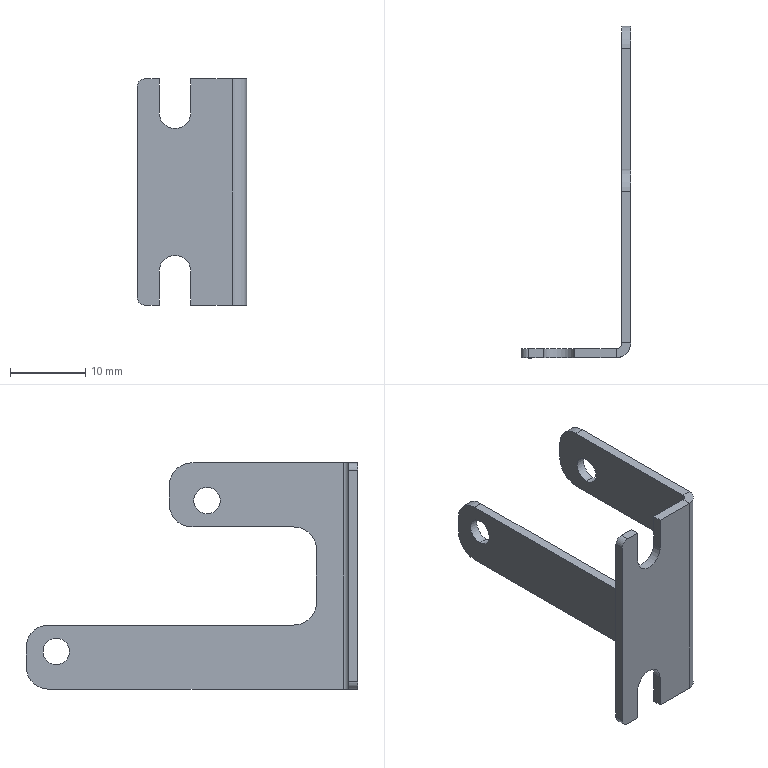Part | SolidWorks | features ICE 3, Fillet 2, EdgeFlange 1, FlatPattern 1, MirrorPattern 1, SMBaseFlange 1, SheetMetal 1 | 1 solid | 38 faces | box 14.5 x 44 x 30 mm | volume 1158 mm3 | plane 22 | cylinder 16 | commonest cylinder face diameters 6 x6 3.5 x4 2 x2 4.2 x2 1.473 x1 3.873 x1
STEP:
#1=CARTESIAN_POINT('',(-1.2,18.,-11.75));
#2=VERTEX_POINT('',#1);
#3=CARTESIAN_POINT('',(-1.2,18.,-8.25));
#4=VERTEX_POINT('',#3);
#5=CARTESIAN_POINT('',(-1.2,18.,-10.));
#6=DIRECTION('',(-1.,0.,0.));
#7=DIRECTION('',(0.,0.,1.));
#8=AXIS2_PLACEMENT_3D('',#5,#6,#7);
#9=CIRCLE('',#8,1.75);
#10=EDGE_CURVE('',#2,#4,#9,.T.);
#11=ORIENTED_EDGE('',*,*,#10,.T.);
#12=CARTESIAN_POINT('',(0.,18.,-8.25));
#13=VERTEX_POINT('',#12);
#14=CARTESIAN_POINT('',(-10.,18.,-8.25));
#15=DIRECTION('',(1.,0.,0.));
#16=VECTOR('',#15,1000.);
#17=LINE('',#14,#16);
#18=EDGE_CURVE('',#4,#13,#17,.T.);
#19=ORIENTED_EDGE('',*,*,#18,.T.);
#20=CARTESIAN_POINT('',(0.,18.,-11.75));
#21=VERTEX_POINT('',#20);
#22=CARTESIAN_POINT('',(0.,18.,-10.));
#23=DIRECTION('',(1.,0.,0.));
#24=DIRECTION('',(0.,0.,-1.));
#25=AXIS2_PLACEMENT_3D('',#22,#23,#24);
#26=CIRCLE('',#25,1.75);
#27=EDGE_CURVE('',#13,#21,#26,.T.);
#28=ORIENTED_EDGE('',*,*,#27,.T.);
#29=CARTESIAN_POINT('',(-10.,18.,-11.75));
#30=DIRECTION('',(1.,0.,0.));
#31=VECTOR('',#30,1000.);
#32=LINE('',#29,#31);
#33=EDGE_CURVE('',#2,#21,#32,.T.);
#34=ORIENTED_EDGE('',*,*,#33,.F.);
#35=EDGE_LOOP('',(#11,#19,#28,#34));
#36=FACE_OUTER_BOUND('',#35,.T.);
#37=CARTESIAN_POINT('',(-10.,18.,-10.));
#38=DIRECTION('',(1.,0.,0.));
#39=DIRECTION('',(0.,0.,-1.));
#40=AXIS2_PLACEMENT_3D('',#37,#38,#39);
#41=CYLINDRICAL_SURFACE('',#40,1.75);
#42=ADVANCED_FACE('',(#36),#41,.F.);
#43=CARTESIAN_POINT('',(-1.2,-2.,8.25));
#44=VERTEX_POINT('',#43);
#45=CARTESIAN_POINT('',(-1.2,-2.,11.75));
#46=VERTEX_POINT('',#45);
#47=CARTESIAN_POINT('',(-1.2,-2.,10.));
#48=DIRECTION('',(-1.,0.,0.));
#49=DIRECTION('',(0.,0.,1.));
#50=AXIS2_PLACEMENT_3D('',#47,#48,#49);
#51=CIRCLE('',#50,1.75);
#52=EDGE_CURVE('',#44,#46,#51,.T.);
#53=ORIENTED_EDGE('',*,*,#52,.T.);
#54=CARTESIAN_POINT('',(0.,-2.,11.75));
#55=VERTEX_POINT('',#54);
#56=CARTESIAN_POINT('',(-10.,-2.,11.75));
#57=DIRECTION('',(1.,0.,0.));
#58=VECTOR('',#57,1000.);
#59=LINE('',#56,#58);
#60=EDGE_CURVE('',#46,#55,#59,.T.);
#61=ORIENTED_EDGE('',*,*,#60,.T.);
#62=CARTESIAN_POINT('',(0.,-2.,8.25));
#63=VERTEX_POINT('',#62);
#64=CARTESIAN_POINT('',(0.,-2.,10.));
#65=DIRECTION('',(1.,0.,0.));
#66=DIRECTION('',(0.,0.,-1.));
#67=AXIS2_PLACEMENT_3D('',#64,#65,#66);
#68=CIRCLE('',#67,1.75);
#69=EDGE_CURVE('',#55,#63,#68,.T.);
#70=ORIENTED_EDGE('',*,*,#69,.T.);
#71=CARTESIAN_POINT('',(-10.,-2.,8.25));
#72=DIRECTION('',(1.,0.,0.));
#73=VECTOR('',#72,1000.);
#74=LINE('',#71,#73);
#75=EDGE_CURVE('',#44,#63,#74,.T.);
#76=ORIENTED_EDGE('',*,*,#75,.F.);
#77=EDGE_LOOP('',(#53,#61,#70,#76));
#78=FACE_OUTER_BOUND('',#77,.T.);
#79=CARTESIAN_POINT('',(-10.,-2.,10.));
#80=DIRECTION('',(1.,0.,0.));
#81=DIRECTION('',(0.,0.,-1.));
#82=AXIS2_PLACEMENT_3D('',#79,#80,#81);
#83=CYLINDRICAL_SURFACE('',#82,1.75);
#84=ADVANCED_FACE('',(#78),#83,.F.);
#85=CARTESIAN_POINT('',(-7.4,-20.8,15.));
#86=VERTEX_POINT('',#85);
#87=CARTESIAN_POINT('',(-1.937,-20.8,15.));
#88=VERTEX_POINT('',#87);
#89=CARTESIAN_POINT('',(-1.2,-20.8,15.));
#90=DIRECTION('',(1.,0.,0.));
#91=VECTOR('',#90,1000.);
#92=LINE('',#89,#91);
#93=EDGE_CURVE('',#86,#88,#92,.T.);
#94=ORIENTED_EDGE('',*,*,#93,.F.);
#95=CARTESIAN_POINT('',(-7.4,-22.,15.));
#96=VERTEX_POINT('',#95);
#97=CARTESIAN_POINT('',(-7.4,-30.8,15.));
#98=DIRECTION('',(0.,1.,0.));
#99=VECTOR('',#98,1000.);
#100=LINE('',#97,#99);
#101=EDGE_CURVE('',#96,#86,#100,.T.);
#102=ORIENTED_EDGE('',*,*,#101,.F.);
#103=CARTESIAN_POINT('',(-1.937,-22.,15.));
#104=VERTEX_POINT('',#103);
#105=CARTESIAN_POINT('',(-1.2,-22.,15.));
#106=DIRECTION('',(1.,0.,0.));
#107=VECTOR('',#106,1000.);
#108=LINE('',#105,#107);
#109=EDGE_CURVE('',#96,#104,#108,.T.);
#110=ORIENTED_EDGE('',*,*,#109,.T.);
#111=CARTESIAN_POINT('',(-1.937,-20.8,15.));
#112=DIRECTION('',(0.,-1.,0.));
#113=VECTOR('',#112,1000.);
#114=LINE('',#111,#113);
#115=EDGE_CURVE('',#88,#104,#114,.T.);
#116=ORIENTED_EDGE('',*,*,#115,.F.);
#117=EDGE_LOOP('',(#94,#102,#110,#116));
#118=FACE_OUTER_BOUND('',#117,.T.);
#119=CARTESIAN_POINT('',(-1.2,-22.,15.));
#120=DIRECTION('',(0.,0.,1.));
#121=DIRECTION('',(1.,0.,0.));
#122=AXIS2_PLACEMENT_3D('',#119,#120,#121);
#123=PLANE('',#122);
#124=ADVANCED_FACE('',(#118),#123,.T.);
#125=CARTESIAN_POINT('',(-13.5,-22.,15.));
#126=VERTEX_POINT('',#125);
#127=CARTESIAN_POINT('',(-11.6,-22.,15.));
#128=VERTEX_POINT('',#127);
#129=CARTESIAN_POINT('',(-1.2,-22.,15.));
#130=DIRECTION('',(1.,0.,0.));
#131=VECTOR('',#130,1000.);
#132=LINE('',#129,#131);
#133=EDGE_CURVE('',#126,#128,#132,.T.);
#134=ORIENTED_EDGE('',*,*,#133,.T.);
#135=CARTESIAN_POINT('',(-11.6,-20.8,15.));
#136=VERTEX_POINT('',#135);
#137=CARTESIAN_POINT('',(-11.6,-30.8,15.));
#138=DIRECTION('',(0.,1.,0.));
#139=VECTOR('',#138,1000.);
#140=LINE('',#137,#139);
#141=EDGE_CURVE('',#128,#136,#140,.T.);
#142=ORIENTED_EDGE('',*,*,#141,.T.);
#143=CARTESIAN_POINT('',(-13.5,-20.8,15.));
#144=VERTEX_POINT('',#143);
#145=CARTESIAN_POINT('',(-1.2,-20.8,15.));
#146=DIRECTION('',(1.,0.,0.));
#147=VECTOR('',#146,1000.);
#148=LINE('',#145,#147);
#149=EDGE_CURVE('',#144,#136,#148,.T.);
#150=ORIENTED_EDGE('',*,*,#149,.F.);
#151=CARTESIAN_POINT('',(-13.5,-22.,15.));
#152=DIRECTION('',(0.,-1.,0.));
#153=VECTOR('',#152,1000.);
#154=LINE('',#151,#153);
#155=EDGE_CURVE('',#144,#126,#154,.T.);
#156=ORIENTED_EDGE('',*,*,#155,.T.);
#157=EDGE_LOOP('',(#134,#142,#150,#156));
#158=FACE_OUTER_BOUND('',#157,.T.);
#159=CARTESIAN_POINT('',(-1.2,-22.,15.));
#160=DIRECTION('',(0.,0.,1.));
#161=DIRECTION('',(1.,0.,0.));
#162=AXIS2_PLACEMENT_3D('',#159,#160,#161);
#163=PLANE('',#162);
#164=ADVANCED_FACE('',(#158),#163,.T.);
#165=ORIENTED_EDGE('',*,*,#109,.F.);
#166=CARTESIAN_POINT('',(-7.4,-22.,10.5));
#167=VERTEX_POINT('',#166);
#168=CARTESIAN_POINT('',(-7.4,-22.,15.));
#169=DIRECTION('',(0.,0.,-1.));
#170=VECTOR('',#169,1000.);
#171=LINE('',#168,#170);
#172=EDGE_CURVE('',#96,#167,#171,.T.);
#173=ORIENTED_EDGE('',*,*,#172,.T.);
#174=CARTESIAN_POINT('',(-11.6,-22.,10.5));
#175=VERTEX_POINT('',#174);
#176=CARTESIAN_POINT('',(-9.5,-22.,10.5));
#177=DIRECTION('',(0.,1.,0.));
#178=DIRECTION('',(1.,0.,0.));
#179=AXIS2_PLACEMENT_3D('',#176,#177,#178);
#180=CIRCLE('',#179,2.1);
#181=EDGE_CURVE('',#167,#175,#180,.T.);
#182=ORIENTED_EDGE('',*,*,#181,.T.);
#183=CARTESIAN_POINT('',(-11.6,-22.,15.));
#184=DIRECTION('',(0.,0.,1.));
#185=VECTOR('',#184,1000.);
#186=LINE('',#183,#185);
#187=EDGE_CURVE('',#175,#128,#186,.T.);
#188=ORIENTED_EDGE('',*,*,#187,.T.);
#189=ORIENTED_EDGE('',*,*,#133,.F.);
#190=CARTESIAN_POINT('',(-14.5,-22.,14.));
#191=VERTEX_POINT('',#190);
#192=CARTESIAN_POINT('',(-13.5,-22.,14.));
#193=DIRECTION('',(0.,-1.,0.));
#194=DIRECTION('',(1.,0.,0.));
#195=AXIS2_PLACEMENT_3D('',#192,#193,#194);
#196=CIRCLE('',#195,1.);
#197=EDGE_CURVE('',#126,#191,#196,.T.);
#198=ORIENTED_EDGE('',*,*,#197,.T.);
#199=CARTESIAN_POINT('',(-14.5,-22.,-14.));
#200=VERTEX_POINT('',#199);
#201=CARTESIAN_POINT('',(-14.5,-22.,15.));
#202=DIRECTION('',(0.,0.,1.));
#203=VECTOR('',#202,1000.);
#204=LINE('',#201,#203);
#205=EDGE_CURVE('',#200,#191,#204,.T.);
#206=ORIENTED_EDGE('',*,*,#205,.F.);
#207=CARTESIAN_POINT('',(-13.5,-22.,-15.));
#208=VERTEX_POINT('',#207);
#209=CARTESIAN_POINT('',(-13.5,-22.,-14.));
#210=DIRECTION('',(0.,-1.,0.));
#211=DIRECTION('',(1.,0.,0.));
#212=AXIS2_PLACEMENT_3D('',#209,#210,#211);
#213=CIRCLE('',#212,1.);
#214=EDGE_CURVE('',#200,#208,#213,.T.);
#215=ORIENTED_EDGE('',*,*,#214,.T.);
#216=CARTESIAN_POINT('',(-11.6,-22.,-15.));
#217=VERTEX_POINT('',#216);
#218=CARTESIAN_POINT('',(-14.5,-22.,-15.));
#219=DIRECTION('',(-1.,0.,0.));
#220=VECTOR('',#219,1000.);
#221=LINE('',#218,#220);
#222=EDGE_CURVE('',#217,#208,#221,.T.);
#223=ORIENTED_EDGE('',*,*,#222,.F.);
#224=CARTESIAN_POINT('',(-11.6,-22.,-10.5));
#225=VERTEX_POINT('',#224);
#226=CARTESIAN_POINT('',(-11.6,-22.,15.));
#227=DIRECTION('',(0.,0.,-1.));
#228=VECTOR('',#227,1000.);
#229=LINE('',#226,#228);
#230=EDGE_CURVE('',#225,#217,#229,.T.);
#231=ORIENTED_EDGE('',*,*,#230,.F.);
#232=CARTESIAN_POINT('',(-7.4,-22.,-10.5));
#233=VERTEX_POINT('',#232);
#234=CARTESIAN_POINT('',(-9.5,-22.,-10.5));
#235=DIRECTION('',(0.,-1.,0.));
#236=DIRECTION('',(1.,0.,0.));
#237=AXIS2_PLACEMENT_3D('',#234,#235,#236);
#238=CIRCLE('',#237,2.1);
#239=EDGE_CURVE('',#233,#225,#238,.T.);
#240=ORIENTED_EDGE('',*,*,#239,.F.);
#241=CARTESIAN_POINT('',(-7.4,-22.,-15.));
#242=VERTEX_POINT('',#241);
#243=CARTESIAN_POINT('',(-7.4,-22.,15.));
#244=DIRECTION('',(0.,0.,1.));
#245=VECTOR('',#244,1000.);
#246=LINE('',#243,#245);
#247=EDGE_CURVE('',#242,#233,#246,.T.);
#248=ORIENTED_EDGE('',*,*,#247,.F.);
#249=CARTESIAN_POINT('',(-1.937,-22.,-15.));
#250=VERTEX_POINT('',#249);
#251=CARTESIAN_POINT('',(-14.5,-22.,-15.));
#252=DIRECTION('',(-1.,0.,0.));
#253=VECTOR('',#252,1000.);
#254=LINE('',#251,#253);
#255=EDGE_CURVE('',#250,#242,#254,.T.);
#256=ORIENTED_EDGE('',*,*,#255,.F.);
#257=CARTESIAN_POINT('',(-1.937,-22.,15.));
#258=DIRECTION('',(0.,0.,1.));
#259=VECTOR('',#258,1000.);
#260=LINE('',#257,#259);
#261=EDGE_CURVE('',#250,#104,#260,.T.);
#262=ORIENTED_EDGE('',*,*,#261,.T.);
#263=EDGE_LOOP('',(#165,#173,#182,#188,#189,#198,#206,#215,#223,#231,#240,#248,#256,#262));
#264=FACE_OUTER_BOUND('',#263,.T.);
#265=CARTESIAN_POINT('',(-1.2,-22.,15.));
#266=DIRECTION('',(0.,-1.,0.));
#267=DIRECTION('',(1.,0.,0.));
#268=AXIS2_PLACEMENT_3D('',#265,#266,#267);
#269=PLANE('',#268);
#270=ADVANCED_FACE('',(#264),#269,.T.);
#271=CARTESIAN_POINT('',(-7.4,-20.8,10.5));
#272=VERTEX_POINT('',#271);
#273=CARTESIAN_POINT('',(-7.4,-20.8,15.));
#274=DIRECTION('',(0.,0.,1.));
#275=VECTOR('',#274,1000.);
#276=LINE('',#273,#275);
#277=EDGE_CURVE('',#272,#86,#276,.T.);
#278=ORIENTED_EDGE('',*,*,#277,.T.);
#279=ORIENTED_EDGE('',*,*,#93,.T.);
#280=CARTESIAN_POINT('',(-1.937,-20.8,-15.));
#281=VERTEX_POINT('',#280);
#282=CARTESIAN_POINT('',(-1.937,-20.8,-15.));
#283=DIRECTION('',(0.,0.,1.));
#284=VECTOR('',#283,1000.);
#285=LINE('',#282,#284);
#286=EDGE_CURVE('',#281,#88,#285,.T.);
#287=ORIENTED_EDGE('',*,*,#286,.F.);
#288=CARTESIAN_POINT('',(-7.4,-20.8,-15.));
#289=VERTEX_POINT('',#288);
#290=CARTESIAN_POINT('',(-1.2,-20.8,-15.));
#291=DIRECTION('',(-1.,0.,0.));
#292=VECTOR('',#291,1000.);
#293=LINE('',#290,#292);
#294=EDGE_CURVE('',#281,#289,#293,.T.);
#295=ORIENTED_EDGE('',*,*,#294,.T.);
#296=CARTESIAN_POINT('',(-7.4,-20.8,-10.5));
#297=VERTEX_POINT('',#296);
#298=CARTESIAN_POINT('',(-7.4,-20.8,-15.));
#299=DIRECTION('',(0.,0.,-1.));
#300=VECTOR('',#299,1000.);
#301=LINE('',#298,#300);
#302=EDGE_CURVE('',#297,#289,#301,.T.);
#303=ORIENTED_EDGE('',*,*,#302,.F.);
#304=CARTESIAN_POINT('',(-11.6,-20.8,-10.5));
#305=VERTEX_POINT('',#304);
#306=CARTESIAN_POINT('',(-9.5,-20.8,-10.5));
#307=DIRECTION('',(0.,1.,0.));
#308=DIRECTION('',(1.,0.,0.));
#309=AXIS2_PLACEMENT_3D('',#306,#307,#308);
#310=CIRCLE('',#309,2.1);
#311=EDGE_CURVE('',#305,#297,#310,.T.);
#312=ORIENTED_EDGE('',*,*,#311,.F.);
#313=CARTESIAN_POINT('',(-11.6,-20.8,-15.));
#314=VERTEX_POINT('',#313);
#315=CARTESIAN_POINT('',(-11.6,-20.8,-15.));
#316=DIRECTION('',(0.,0.,1.));
#317=VECTOR('',#316,1000.);
#318=LINE('',#315,#317);
#319=EDGE_CURVE('',#314,#305,#318,.T.);
#320=ORIENTED_EDGE('',*,*,#319,.F.);
#321=CARTESIAN_POINT('',(-13.5,-20.8,-15.));
#322=VERTEX_POINT('',#321);
#323=CARTESIAN_POINT('',(-1.2,-20.8,-15.));
#324=DIRECTION('',(-1.,0.,0.));
#325=VECTOR('',#324,1000.);
#326=LINE('',#323,#325);
#327=EDGE_CURVE('',#314,#322,#326,.T.);
#328=ORIENTED_EDGE('',*,*,#327,.T.);
#329=CARTESIAN_POINT('',(-14.5,-20.8,-14.));
#330=VERTEX_POINT('',#329);
#331=CARTESIAN_POINT('',(-13.5,-20.8,-14.));
#332=DIRECTION('',(0.,1.,0.));
#333=DIRECTION('',(1.,0.,0.));
#334=AXIS2_PLACEMENT_3D('',#331,#332,#333);
#335=CIRCLE('',#334,1.);
#336=EDGE_CURVE('',#322,#330,#335,.T.);
#337=ORIENTED_EDGE('',*,*,#336,.T.);
#338=CARTESIAN_POINT('',(-14.5,-20.8,14.));
#339=VERTEX_POINT('',#338);
#340=CARTESIAN_POINT('',(-14.5,-20.8,15.));
#341=DIRECTION('',(0.,0.,1.));
#342=VECTOR('',#341,1000.);
#343=LINE('',#340,#342);
#344=EDGE_CURVE('',#330,#339,#343,.T.);
#345=ORIENTED_EDGE('',*,*,#344,.T.);
#346=CARTESIAN_POINT('',(-13.5,-20.8,14.));
#347=DIRECTION('',(0.,1.,0.));
#348=DIRECTION('',(1.,0.,0.));
#349=AXIS2_PLACEMENT_3D('',#346,#347,#348);
#350=CIRCLE('',#349,1.);
#351=EDGE_CURVE('',#339,#144,#350,.T.);
#352=ORIENTED_EDGE('',*,*,#351,.T.);
#353=ORIENTED_EDGE('',*,*,#149,.T.);
#354=CARTESIAN_POINT('',(-11.6,-20.8,10.5));
#355=VERTEX_POINT('',#354);
#356=CARTESIAN_POINT('',(-11.6,-20.8,15.));
#357=DIRECTION('',(0.,0.,-1.));
#358=VECTOR('',#357,1000.);
#359=LINE('',#356,#358);
#360=EDGE_CURVE('',#136,#355,#359,.T.);
#361=ORIENTED_EDGE('',*,*,#360,.T.);
#362=CARTESIAN_POINT('',(-9.5,-20.8,10.5));
#363=DIRECTION('',(0.,-1.,0.));
#364=DIRECTION('',(1.,0.,0.));
#365=AXIS2_PLACEMENT_3D('',#362,#363,#364);
#366=CIRCLE('',#365,2.1);
#367=EDGE_CURVE('',#355,#272,#366,.T.);
#368=ORIENTED_EDGE('',*,*,#367,.T.);
#369=EDGE_LOOP('',(#278,#279,#287,#295,#303,#312,#320,#328,#337,#345,#352,#353,#361,#368));
#370=FACE_OUTER_BOUND('',#369,.T.);
#371=CARTESIAN_POINT('',(-1.2,-20.8,15.));
#372=DIRECTION('',(0.,-1.,0.));
#373=DIRECTION('',(1.,0.,0.));
#374=AXIS2_PLACEMENT_3D('',#371,#372,#373);
#375=PLANE('',#374);
#376=ADVANCED_FACE('',(#370),#375,.F.);
#377=CARTESIAN_POINT('',(-7.4,-30.8,-15.));
#378=DIRECTION('',(0.,1.,0.));
#379=VECTOR('',#378,1000.);
#380=LINE('',#377,#379);
#381=EDGE_CURVE('',#242,#289,#380,.T.);
#382=ORIENTED_EDGE('',*,*,#381,.T.);
#383=ORIENTED_EDGE('',*,*,#294,.F.);
#384=CARTESIAN_POINT('',(-1.937,-22.,-15.));
#385=DIRECTION('',(0.,-1.,0.));
#386=VECTOR('',#385,1000.);
#387=LINE('',#384,#386);
#388=EDGE_CURVE('',#281,#250,#387,.T.);
#389=ORIENTED_EDGE('',*,*,#388,.T.);
#390=ORIENTED_EDGE('',*,*,#255,.T.);
#391=EDGE_LOOP('',(#382,#383,#389,#390));
#392=FACE_OUTER_BOUND('',#391,.T.);
#393=CARTESIAN_POINT('',(-14.5,-22.,-15.));
#394=DIRECTION('',(0.,0.,-1.));
#395=DIRECTION('',(-1.,0.,0.));
#396=AXIS2_PLACEMENT_3D('',#393,#394,#395);
#397=PLANE('',#396);
#398=ADVANCED_FACE('',(#392),#397,.T.);
#399=CARTESIAN_POINT('',(-1.2,0.,15.));
#400=VERTEX_POINT('',#399);
#401=CARTESIAN_POINT('',(-1.2,-20.063,15.));
#402=VERTEX_POINT('',#401);
#403=CARTESIAN_POINT('',(-1.2,-22.,15.));
#404=DIRECTION('',(0.,-1.,0.));
#405=VECTOR('',#404,1000.);
#406=LINE('',#403,#405);
#407=EDGE_CURVE('',#400,#402,#406,.T.);
#408=ORIENTED_EDGE('',*,*,#407,.T.);
#409=CARTESIAN_POINT('',(0.,-20.063,15.));
#410=VERTEX_POINT('',#409);
#411=CARTESIAN_POINT('',(-1.2,-20.063,15.));
#412=DIRECTION('',(1.,0.,0.));
#413=VECTOR('',#412,1000.);
#414=LINE('',#411,#413);
#415=EDGE_CURVE('',#402,#410,#414,.T.);
#416=ORIENTED_EDGE('',*,*,#415,.T.);
#417=CARTESIAN_POINT('',(0.,0.,15.));
#418=VERTEX_POINT('',#417);
#419=CARTESIAN_POINT('',(0.,-22.,15.));
#420=DIRECTION('',(0.,-1.,0.));
#421=VECTOR('',#420,1000.);
#422=LINE('',#419,#421);
#423=EDGE_CURVE('',#418,#410,#422,.T.);
#424=ORIENTED_EDGE('',*,*,#423,.F.);
#425=CARTESIAN_POINT('',(-1.2,0.,15.));
#426=DIRECTION('',(-1.,0.,0.));
#427=VECTOR('',#426,1000.);
#428=LINE('',#425,#427);
#429=EDGE_CURVE('',#418,#400,#428,.T.);
#430=ORIENTED_EDGE('',*,*,#429,.T.);
#431=EDGE_LOOP('',(#408,#416,#424,#430));
#432=FACE_OUTER_BOUND('',#431,.T.);
#433=CARTESIAN_POINT('',(-1.2,-22.,15.));
#434=DIRECTION('',(0.,0.,1.));
#435=DIRECTION('',(1.,0.,0.));
#436=AXIS2_PLACEMENT_3D('',#433,#434,#435);
#437=PLANE('',#436);
#438=ADVANCED_FACE('',(#432),#437,.T.);
#439=ORIENTED_EDGE('',*,*,#10,.F.);
#440=CARTESIAN_POINT('',(-1.2,18.,-10.));
#441=DIRECTION('',(-1.,0.,0.));
#442=DIRECTION('',(0.,0.,1.));
#443=AXIS2_PLACEMENT_3D('',#440,#441,#442);
#444=CIRCLE('',#443,1.75);
#445=EDGE_CURVE('',#4,#2,#444,.T.);
#446=ORIENTED_EDGE('',*,*,#445,.F.);
#447=EDGE_LOOP('',(#439,#446));
#448=FACE_BOUND('',#447,.T.);
#449=ORIENTED_EDGE('',*,*,#52,.F.);
#450=CARTESIAN_POINT('',(-1.2,-2.,10.));
#451=DIRECTION('',(-1.,0.,0.));
#452=DIRECTION('',(0.,0.,1.));
#453=AXIS2_PLACEMENT_3D('',#450,#451,#452);
#454=CIRCLE('',#453,1.75);
#455=EDGE_CURVE('',#46,#44,#454,.T.);
#456=ORIENTED_EDGE('',*,*,#455,.F.);
#457=EDGE_LOOP('',(#449,#456));
#458=FACE_BOUND('',#457,.T.);
#459=CARTESIAN_POINT('',(-1.2,-20.063,-15.));
#460=VERTEX_POINT('',#459);
#461=CARTESIAN_POINT('',(-1.2,19.,-15.));
#462=VERTEX_POINT('',#461);
#463=CARTESIAN_POINT('',(-1.2,-22.,-15.));
#464=DIRECTION('',(0.,1.,0.));
#465=VECTOR('',#464,1000.);
#466=LINE('',#463,#465);
#467=EDGE_CURVE('',#460,#462,#466,.T.);
#468=ORIENTED_EDGE('',*,*,#467,.F.);
#469=CARTESIAN_POINT('',(-1.2,-20.063,15.));
#470=DIRECTION('',(0.,0.,-1.));
#471=VECTOR('',#470,1000.);
#472=LINE('',#469,#471);
#473=EDGE_CURVE('',#402,#460,#472,.T.);
#474=ORIENTED_EDGE('',*,*,#473,.F.);
#475=ORIENTED_EDGE('',*,*,#407,.F.);
#476=CARTESIAN_POINT('',(-1.2,3.,12.));
#477=VERTEX_POINT('',#476);
#478=CARTESIAN_POINT('',(-1.2,0.,12.));
#479=DIRECTION('',(-1.,0.,0.));
#480=DIRECTION('',(0.,0.,1.));
#481=AXIS2_PLACEMENT_3D('',#478,#479,#480);
#482=CIRCLE('',#481,3.);
#483=EDGE_CURVE('',#400,#477,#482,.T.);
#484=ORIENTED_EDGE('',*,*,#483,.T.);
#485=CARTESIAN_POINT('',(-1.2,3.,9.5));
#486=VERTEX_POINT('',#485);
#487=CARTESIAN_POINT('',(-1.2,3.,6.5));
#488=DIRECTION('',(0.,0.,-1.));
#489=VECTOR('',#488,1000.);
#490=LINE('',#487,#489);
#491=EDGE_CURVE('',#477,#486,#490,.T.);
#492=ORIENTED_EDGE('',*,*,#491,.T.);
#493=CARTESIAN_POINT('',(-1.2,0.,6.5));
#494=VERTEX_POINT('',#493);
#495=CARTESIAN_POINT('',(-1.2,0.,9.5));
#496=DIRECTION('',(-1.,0.,0.));
#497=DIRECTION('',(0.,0.,1.));
#498=AXIS2_PLACEMENT_3D('',#495,#496,#497);
#499=CIRCLE('',#498,3.);
#500=EDGE_CURVE('',#486,#494,#499,.T.);
#501=ORIENTED_EDGE('',*,*,#500,.T.);
#502=CARTESIAN_POINT('',(-1.2,-13.5,6.5));
#503=VERTEX_POINT('',#502);
#504=CARTESIAN_POINT('',(-1.2,3.,6.5));
#505=DIRECTION('',(0.,-1.,0.));
#506=VECTOR('',#505,1000.);
#507=LINE('',#504,#506);
#508=EDGE_CURVE('',#494,#503,#507,.T.);
#509=ORIENTED_EDGE('',*,*,#508,.T.);
#510=CARTESIAN_POINT('',(-1.2,-16.5,3.5));
#511=VERTEX_POINT('',#510);
#512=CARTESIAN_POINT('',(-1.2,-13.5,3.5));
#513=DIRECTION('',(1.,0.,0.));
#514=DIRECTION('',(0.,0.,1.));
#515=AXIS2_PLACEMENT_3D('',#512,#513,#514);
#516=CIRCLE('',#515,3.);
#517=EDGE_CURVE('',#503,#511,#516,.T.);
#518=ORIENTED_EDGE('',*,*,#517,.T.);
#519=CARTESIAN_POINT('',(-1.2,-16.5,-3.5));
#520=VERTEX_POINT('',#519);
#521=CARTESIAN_POINT('',(-1.2,-16.5,-6.5));
#522=DIRECTION('',(0.,0.,-1.));
#523=VECTOR('',#522,1000.);
#524=LINE('',#521,#523);
#525=EDGE_CURVE('',#511,#520,#524,.T.);
#526=ORIENTED_EDGE('',*,*,#525,.T.);
#527=CARTESIAN_POINT('',(-1.2,-13.5,-6.5));
#528=VERTEX_POINT('',#527);
#529=CARTESIAN_POINT('',(-1.2,-13.5,-3.5));
#530=DIRECTION('',(1.,0.,0.));
#531=DIRECTION('',(0.,0.,1.));
#532=AXIS2_PLACEMENT_3D('',#529,#530,#531);
#533=CIRCLE('',#532,3.);
#534=EDGE_CURVE('',#520,#528,#533,.T.);
#535=ORIENTED_EDGE('',*,*,#534,.T.);
#536=CARTESIAN_POINT('',(-1.2,19.,-6.5));
#537=VERTEX_POINT('',#536);
#538=CARTESIAN_POINT('',(-1.2,22.,-6.5));
#539=DIRECTION('',(0.,1.,0.));
#540=VECTOR('',#539,1000.);
#541=LINE('',#538,#540);
#542=EDGE_CURVE('',#528,#537,#541,.T.);
#543=ORIENTED_EDGE('',*,*,#542,.T.);
#544=CARTESIAN_POINT('',(-1.2,22.,-9.5));
#545=VERTEX_POINT('',#544);
#546=CARTESIAN_POINT('',(-1.2,19.,-9.5));
#547=DIRECTION('',(-1.,0.,0.));
#548=DIRECTION('',(0.,0.,1.));
#549=AXIS2_PLACEMENT_3D('',#546,#547,#548);
#550=CIRCLE('',#549,3.);
#551=EDGE_CURVE('',#537,#545,#550,.T.);
#552=ORIENTED_EDGE('',*,*,#551,.T.);
#553=CARTESIAN_POINT('',(-1.2,22.,-12.));
#554=VERTEX_POINT('',#553);
#555=CARTESIAN_POINT('',(-1.2,22.,15.));
#556=DIRECTION('',(0.,0.,1.));
#557=VECTOR('',#556,1000.);
#558=LINE('',#555,#557);
#559=EDGE_CURVE('',#554,#545,#558,.T.);
#560=ORIENTED_EDGE('',*,*,#559,.F.);
#561=CARTESIAN_POINT('',(-1.2,19.,-12.));
#562=DIRECTION('',(-1.,0.,0.));
#563=DIRECTION('',(0.,0.,1.));
#564=AXIS2_PLACEMENT_3D('',#561,#562,#563);
#565=CIRCLE('',#564,3.);
#566=EDGE_CURVE('',#554,#462,#565,.T.);
#567=ORIENTED_EDGE('',*,*,#566,.T.);
#568=EDGE_LOOP('',(#468,#474,#475,#484,#492,#501,#509,#518,#526,#535,#543,#552,#560,#567));
#569=FACE_OUTER_BOUND('',#568,.T.);
#570=CARTESIAN_POINT('',(-1.2,22.,-15.));
#571=DIRECTION('',(-1.,0.,0.));
#572=DIRECTION('',(0.,0.,1.));
#573=AXIS2_PLACEMENT_3D('',#570,#571,#572);
#574=PLANE('',#573);
#575=ADVANCED_FACE('',(#448,#458,#569),#574,.T.);
#576=CARTESIAN_POINT('',(0.,18.,-10.));
#577=DIRECTION('',(1.,0.,0.));
#578=DIRECTION('',(0.,0.,-1.));
#579=AXIS2_PLACEMENT_3D('',#576,#577,#578);
#580=CIRCLE('',#579,1.75);
#581=EDGE_CURVE('',#21,#13,#580,.T.);
#582=ORIENTED_EDGE('',*,*,#581,.F.);
#583=ORIENTED_EDGE('',*,*,#27,.F.);
#584=EDGE_LOOP('',(#582,#583));
#585=FACE_BOUND('',#584,.T.);
#586=CARTESIAN_POINT('',(0.,-2.,10.));
#587=DIRECTION('',(1.,0.,0.));
#588=DIRECTION('',(0.,0.,-1.));
#589=AXIS2_PLACEMENT_3D('',#586,#587,#588);
#590=CIRCLE('',#589,1.75);
#591=EDGE_CURVE('',#63,#55,#590,.T.);
#592=ORIENTED_EDGE('',*,*,#591,.F.);
#593=ORIENTED_EDGE('',*,*,#69,.F.);
#594=EDGE_LOOP('',(#592,#593));
#595=FACE_BOUND('',#594,.T.);
#596=CARTESIAN_POINT('',(0.,-20.063,-15.));
#597=VERTEX_POINT('',#596);
#598=CARTESIAN_POINT('',(0.,-20.063,15.));
#599=DIRECTION('',(0.,0.,-1.));
#600=VECTOR('',#599,1000.);
#601=LINE('',#598,#600);
#602=EDGE_CURVE('',#410,#597,#601,.T.);
#603=ORIENTED_EDGE('',*,*,#602,.T.);
#604=CARTESIAN_POINT('',(0.,19.,-15.));
#605=VERTEX_POINT('',#604);
#606=CARTESIAN_POINT('',(0.,-22.,-15.));
#607=DIRECTION('',(0.,1.,0.));
#608=VECTOR('',#607,1000.);
#609=LINE('',#606,#608);
#610=EDGE_CURVE('',#597,#605,#609,.T.);
#611=ORIENTED_EDGE('',*,*,#610,.T.);
#612=CARTESIAN_POINT('',(0.,22.,-12.));
#613=VERTEX_POINT('',#612);
#614=CARTESIAN_POINT('',(0.,19.,-12.));
#615=DIRECTION('',(1.,0.,0.));
#616=DIRECTION('',(0.,0.,1.));
#617=AXIS2_PLACEMENT_3D('',#614,#615,#616);
#618=CIRCLE('',#617,3.);
#619=EDGE_CURVE('',#605,#613,#618,.T.);
#620=ORIENTED_EDGE('',*,*,#619,.T.);
#621=CARTESIAN_POINT('',(0.,22.,-9.5));
#622=VERTEX_POINT('',#621);
#623=CARTESIAN_POINT('',(0.,22.,15.));
#624=DIRECTION('',(0.,0.,1.));
#625=VECTOR('',#624,1000.);
#626=LINE('',#623,#625);
#627=EDGE_CURVE('',#613,#622,#626,.T.);
#628=ORIENTED_EDGE('',*,*,#627,.T.);
#629=CARTESIAN_POINT('',(0.,19.,-6.5));
#630=VERTEX_POINT('',#629);
#631=CARTESIAN_POINT('',(0.,19.,-9.5));
#632=DIRECTION('',(1.,0.,0.));
#633=DIRECTION('',(0.,0.,1.));
#634=AXIS2_PLACEMENT_3D('',#631,#632,#633);
#635=CIRCLE('',#634,3.);
#636=EDGE_CURVE('',#622,#630,#635,.T.);
#637=ORIENTED_EDGE('',*,*,#636,.T.);
#638=CARTESIAN_POINT('',(0.,-13.5,-6.5));
#639=VERTEX_POINT('',#638);
#640=CARTESIAN_POINT('',(0.,22.,-6.5));
#641=DIRECTION('',(0.,1.,0.));
#642=VECTOR('',#641,1000.);
#643=LINE('',#640,#642);
#644=EDGE_CURVE('',#639,#630,#643,.T.);
#645=ORIENTED_EDGE('',*,*,#644,.F.);
#646=CARTESIAN_POINT('',(0.,-16.5,-3.5));
#647=VERTEX_POINT('',#646);
#648=CARTESIAN_POINT('',(0.,-13.5,-3.5));
#649=DIRECTION('',(-1.,0.,0.));
#650=DIRECTION('',(0.,0.,1.));
#651=AXIS2_PLACEMENT_3D('',#648,#649,#650);
#652=CIRCLE('',#651,3.);
#653=EDGE_CURVE('',#639,#647,#652,.T.);
#654=ORIENTED_EDGE('',*,*,#653,.T.);
#655=CARTESIAN_POINT('',(0.,-16.5,3.5));
#656=VERTEX_POINT('',#655);
#657=CARTESIAN_POINT('',(0.,-16.5,-6.5));
#658=DIRECTION('',(0.,0.,-1.));
#659=VECTOR('',#658,1000.);
#660=LINE('',#657,#659);
#661=EDGE_CURVE('',#656,#647,#660,.T.);
#662=ORIENTED_EDGE('',*,*,#661,.F.);
#663=CARTESIAN_POINT('',(0.,-13.5,6.5));
#664=VERTEX_POINT('',#663);
#665=CARTESIAN_POINT('',(0.,-13.5,3.5));
#666=DIRECTION('',(-1.,0.,0.));
#667=DIRECTION('',(0.,0.,1.));
#668=AXIS2_PLACEMENT_3D('',#665,#666,#667);
#669=CIRCLE('',#668,3.);
#670=EDGE_CURVE('',#656,#664,#669,.T.);
#671=ORIENTED_EDGE('',*,*,#670,.T.);
#672=CARTESIAN_POINT('',(0.,0.,6.5));
#673=VERTEX_POINT('',#672);
#674=CARTESIAN_POINT('',(0.,3.,6.5));
#675=DIRECTION('',(0.,-1.,0.));
#676=VECTOR('',#675,1000.);
#677=LINE('',#674,#676);
#678=EDGE_CURVE('',#673,#664,#677,.T.);
#679=ORIENTED_EDGE('',*,*,#678,.F.);
#680=CARTESIAN_POINT('',(0.,3.,9.5));
#681=VERTEX_POINT('',#680);
#682=CARTESIAN_POINT('',(0.,0.,9.5));
#683=DIRECTION('',(1.,0.,0.));
#684=DIRECTION('',(0.,0.,1.));
#685=AXIS2_PLACEMENT_3D('',#682,#683,#684);
#686=CIRCLE('',#685,3.);
#687=EDGE_CURVE('',#673,#681,#686,.T.);
#688=ORIENTED_EDGE('',*,*,#687,.T.);
#689=CARTESIAN_POINT('',(0.,3.,12.));
#690=VERTEX_POINT('',#689);
#691=CARTESIAN_POINT('',(0.,3.,6.5));
#692=DIRECTION('',(0.,0.,-1.));
#693=VECTOR('',#692,1000.);
#694=LINE('',#691,#693);
#695=EDGE_CURVE('',#690,#681,#694,.T.);
#696=ORIENTED_EDGE('',*,*,#695,.F.);
#697=CARTESIAN_POINT('',(0.,0.,12.));
#698=DIRECTION('',(1.,0.,0.));
#699=DIRECTION('',(0.,0.,1.));
#700=AXIS2_PLACEMENT_3D('',#697,#698,#699);
#701=CIRCLE('',#700,3.);
#702=EDGE_CURVE('',#690,#418,#701,.T.);
#703=ORIENTED_EDGE('',*,*,#702,.T.);
#704=ORIENTED_EDGE('',*,*,#423,.T.);
#705=EDGE_LOOP('',(#603,#611,#620,#628,#637,#645,#654,#662,#671,#679,#688,#696,#703,#704));
#706=FACE_OUTER_BOUND('',#705,.T.);
#707=CARTESIAN_POINT('',(0.,22.,-15.));
#708=DIRECTION('',(-1.,0.,0.));
#709=DIRECTION('',(0.,0.,1.));
#710=AXIS2_PLACEMENT_3D('',#707,#708,#709);
#711=PLANE('',#710);
#712=ADVANCED_FACE('',(#585,#595,#706),#711,.F.);
#713=CARTESIAN_POINT('',(-1.2,-20.063,-15.));
#714=DIRECTION('',(1.,0.,0.));
#715=VECTOR('',#714,1000.);
#716=LINE('',#713,#715);
#717=EDGE_CURVE('',#460,#597,#716,.T.);
#718=ORIENTED_EDGE('',*,*,#717,.F.);
#719=ORIENTED_EDGE('',*,*,#467,.T.);
#720=CARTESIAN_POINT('',(-1.2,19.,-15.));
#721=DIRECTION('',(1.,0.,0.));
#722=VECTOR('',#721,1000.);
#723=LINE('',#720,#722);
#724=EDGE_CURVE('',#462,#605,#723,.T.);
#725=ORIENTED_EDGE('',*,*,#724,.T.);
#726=ORIENTED_EDGE('',*,*,#610,.F.);
#727=EDGE_LOOP('',(#718,#719,#725,#726));
#728=FACE_OUTER_BOUND('',#727,.T.);
#729=CARTESIAN_POINT('',(-1.2,-22.,-15.));
#730=DIRECTION('',(0.,0.,-1.));
#731=DIRECTION('',(-1.,0.,0.));
#732=AXIS2_PLACEMENT_3D('',#729,#730,#731);
#733=PLANE('',#732);
#734=ADVANCED_FACE('',(#728),#733,.T.);
#735=ORIENTED_EDGE('',*,*,#627,.F.);
#736=CARTESIAN_POINT('',(-1.2,22.,-12.));
#737=DIRECTION('',(-1.,0.,0.));
#738=VECTOR('',#737,1000.);
#739=LINE('',#736,#738);
#740=EDGE_CURVE('',#613,#554,#739,.T.);
#741=ORIENTED_EDGE('',*,*,#740,.T.);
#742=ORIENTED_EDGE('',*,*,#559,.T.);
#743=CARTESIAN_POINT('',(0.,22.,-9.5));
#744=DIRECTION('',(1.,0.,0.));
#745=VECTOR('',#744,1000.);
#746=LINE('',#743,#745);
#747=EDGE_CURVE('',#545,#622,#746,.T.);
#748=ORIENTED_EDGE('',*,*,#747,.T.);
#749=EDGE_LOOP('',(#735,#741,#742,#748));
#750=FACE_OUTER_BOUND('',#749,.T.);
#751=CARTESIAN_POINT('',(-1.2,22.,15.));
#752=DIRECTION('',(0.,1.,0.));
#753=DIRECTION('',(0.,0.,1.));
#754=AXIS2_PLACEMENT_3D('',#751,#752,#753);
#755=PLANE('',#754);
#756=ADVANCED_FACE('',(#750),#755,.T.);
#757=ORIENTED_EDGE('',*,*,#644,.T.);
#758=CARTESIAN_POINT('',(-1.2,19.,-6.5));
#759=DIRECTION('',(-1.,0.,0.));
#760=VECTOR('',#759,1000.);
#761=LINE('',#758,#760);
#762=EDGE_CURVE('',#630,#537,#761,.T.);
#763=ORIENTED_EDGE('',*,*,#762,.T.);
#764=ORIENTED_EDGE('',*,*,#542,.F.);
#765=CARTESIAN_POINT('',(0.,-13.5,-6.5));
#766=DIRECTION('',(1.,0.,0.));
#767=VECTOR('',#766,1000.);
#768=LINE('',#765,#767);
#769=EDGE_CURVE('',#528,#639,#768,.T.);
#770=ORIENTED_EDGE('',*,*,#769,.T.);
#771=EDGE_LOOP('',(#757,#763,#764,#770));
#772=FACE_OUTER_BOUND('',#771,.T.);
#773=CARTESIAN_POINT('',(-1.2,22.,-6.5));
#774=DIRECTION('',(0.,0.,-1.));
#775=DIRECTION('',(0.,1.,0.));
#776=AXIS2_PLACEMENT_3D('',#773,#774,#775);
#777=PLANE('',#776);
#778=ADVANCED_FACE('',(#772),#777,.F.);
#779=ORIENTED_EDGE('',*,*,#661,.T.);
#780=CARTESIAN_POINT('',(-1.2,-16.5,-3.5));
#781=DIRECTION('',(-1.,0.,0.));
#782=VECTOR('',#781,1000.);
#783=LINE('',#780,#782);
#784=EDGE_CURVE('',#647,#520,#783,.T.);
#785=ORIENTED_EDGE('',*,*,#784,.T.);
#786=ORIENTED_EDGE('',*,*,#525,.F.);
#787=CARTESIAN_POINT('',(0.,-16.5,3.5));
#788=DIRECTION('',(1.,0.,0.));
#789=VECTOR('',#788,1000.);
#790=LINE('',#787,#789);
#791=EDGE_CURVE('',#511,#656,#790,.T.);
#792=ORIENTED_EDGE('',*,*,#791,.T.);
#793=EDGE_LOOP('',(#779,#785,#786,#792));
#794=FACE_OUTER_BOUND('',#793,.T.);
#795=CARTESIAN_POINT('',(-1.2,-16.5,-6.5));
#796=DIRECTION('',(0.,-1.,0.));
#797=DIRECTION('',(0.,0.,-1.));
#798=AXIS2_PLACEMENT_3D('',#795,#796,#797);
#799=PLANE('',#798);
#800=ADVANCED_FACE('',(#794),#799,.F.);
#801=ORIENTED_EDGE('',*,*,#508,.F.);
#802=CARTESIAN_POINT('',(-1.2,0.,6.5));
#803=DIRECTION('',(1.,0.,0.));
#804=VECTOR('',#803,1000.);
#805=LINE('',#802,#804);
#806=EDGE_CURVE('',#494,#673,#805,.T.);
#807=ORIENTED_EDGE('',*,*,#806,.T.);
#808=ORIENTED_EDGE('',*,*,#678,.T.);
#809=CARTESIAN_POINT('',(-1.2,-13.5,6.5));
#810=DIRECTION('',(-1.,0.,0.));
#811=VECTOR('',#810,1000.);
#812=LINE('',#809,#811);
#813=EDGE_CURVE('',#664,#503,#812,.T.);
#814=ORIENTED_EDGE('',*,*,#813,.T.);
#815=EDGE_LOOP('',(#801,#807,#808,#814));
#816=FACE_OUTER_BOUND('',#815,.T.);
#817=CARTESIAN_POINT('',(-1.2,3.,6.5));
#818=DIRECTION('',(0.,0.,1.));
#819=DIRECTION('',(0.,-1.,0.));
#820=AXIS2_PLACEMENT_3D('',#817,#818,#819);
#821=PLANE('',#820);
#822=ADVANCED_FACE('',(#816),#821,.F.);
#823=ORIENTED_EDGE('',*,*,#491,.F.);
#824=CARTESIAN_POINT('',(0.,3.,12.));
#825=DIRECTION('',(1.,0.,0.));
#826=VECTOR('',#825,1000.);
#827=LINE('',#824,#826);
#828=EDGE_CURVE('',#477,#690,#827,.T.);
#829=ORIENTED_EDGE('',*,*,#828,.T.);
#830=ORIENTED_EDGE('',*,*,#695,.T.);
#831=CARTESIAN_POINT('',(-1.2,3.,9.5));
#832=DIRECTION('',(-1.,0.,0.));
#833=VECTOR('',#832,1000.);
#834=LINE('',#831,#833);
#835=EDGE_CURVE('',#681,#486,#834,.T.);
#836=ORIENTED_EDGE('',*,*,#835,.T.);
#837=EDGE_LOOP('',(#823,#829,#830,#836));
#838=FACE_OUTER_BOUND('',#837,.T.);
#839=CARTESIAN_POINT('',(-1.2,3.,6.5));
#840=DIRECTION('',(0.,-1.,0.));
#841=DIRECTION('',(0.,0.,-1.));
#842=AXIS2_PLACEMENT_3D('',#839,#840,#841);
#843=PLANE('',#842);
#844=ADVANCED_FACE('',(#838),#843,.F.);
#845=ORIENTED_EDGE('',*,*,#566,.F.);
#846=ORIENTED_EDGE('',*,*,#740,.F.);
#847=ORIENTED_EDGE('',*,*,#619,.F.);
#848=ORIENTED_EDGE('',*,*,#724,.F.);
#849=EDGE_LOOP('',(#845,#846,#847,#848));
#850=FACE_OUTER_BOUND('',#849,.T.);
#851=CARTESIAN_POINT('',(-1.2,19.,-12.));
#852=DIRECTION('',(1.,0.,0.));
#853=DIRECTION('',(0.,0.,-1.));
#854=AXIS2_PLACEMENT_3D('',#851,#852,#853);
#855=CYLINDRICAL_SURFACE('',#854,3.);
#856=ADVANCED_FACE('',(#850),#855,.T.);
#857=ORIENTED_EDGE('',*,*,#551,.F.);
#858=ORIENTED_EDGE('',*,*,#762,.F.);
#859=ORIENTED_EDGE('',*,*,#636,.F.);
#860=ORIENTED_EDGE('',*,*,#747,.F.);
#861=EDGE_LOOP('',(#857,#858,#859,#860));
#862=FACE_OUTER_BOUND('',#861,.T.);
#863=CARTESIAN_POINT('',(-1.2,19.,-9.5));
#864=DIRECTION('',(-1.,0.,0.));
#865=DIRECTION('',(0.,0.,1.));
#866=AXIS2_PLACEMENT_3D('',#863,#864,#865);
#867=CYLINDRICAL_SURFACE('',#866,3.);
#868=ADVANCED_FACE('',(#862),#867,.T.);
#869=ORIENTED_EDGE('',*,*,#483,.F.);
#870=ORIENTED_EDGE('',*,*,#429,.F.);
#871=ORIENTED_EDGE('',*,*,#702,.F.);
#872=ORIENTED_EDGE('',*,*,#828,.F.);
#873=EDGE_LOOP('',(#869,#870,#871,#872));
#874=FACE_OUTER_BOUND('',#873,.T.);
#875=CARTESIAN_POINT('',(-1.2,0.,12.));
#876=DIRECTION('',(-1.,0.,0.));
#877=DIRECTION('',(0.,0.,1.));
#878=AXIS2_PLACEMENT_3D('',#875,#876,#877);
#879=CYLINDRICAL_SURFACE('',#878,3.);
#880=ADVANCED_FACE('',(#874),#879,.T.);
#881=ORIENTED_EDGE('',*,*,#500,.F.);
#882=ORIENTED_EDGE('',*,*,#835,.F.);
#883=ORIENTED_EDGE('',*,*,#687,.F.);
#884=ORIENTED_EDGE('',*,*,#806,.F.);
#885=EDGE_LOOP('',(#881,#882,#883,#884));
#886=FACE_OUTER_BOUND('',#885,.T.);
#887=CARTESIAN_POINT('',(-1.2,0.,9.5));
#888=DIRECTION('',(1.,0.,0.));
#889=DIRECTION('',(0.,0.,-1.));
#890=AXIS2_PLACEMENT_3D('',#887,#888,#889);
#891=CYLINDRICAL_SURFACE('',#890,3.);
#892=ADVANCED_FACE('',(#886),#891,.T.);
#893=ORIENTED_EDGE('',*,*,#534,.F.);
#894=ORIENTED_EDGE('',*,*,#784,.F.);
#895=ORIENTED_EDGE('',*,*,#653,.F.);
#896=ORIENTED_EDGE('',*,*,#769,.F.);
#897=EDGE_LOOP('',(#893,#894,#895,#896));
#898=FACE_OUTER_BOUND('',#897,.T.);
#899=CARTESIAN_POINT('',(-1.2,-13.5,-3.5));
#900=DIRECTION('',(-1.,0.,0.));
#901=DIRECTION('',(0.,0.,1.));
#902=AXIS2_PLACEMENT_3D('',#899,#900,#901);
#903=CYLINDRICAL_SURFACE('',#902,3.);
#904=ADVANCED_FACE('',(#898),#903,.F.);
#905=ORIENTED_EDGE('',*,*,#517,.F.);
#906=ORIENTED_EDGE('',*,*,#813,.F.);
#907=ORIENTED_EDGE('',*,*,#670,.F.);
#908=ORIENTED_EDGE('',*,*,#791,.F.);
#909=EDGE_LOOP('',(#905,#906,#907,#908));
#910=FACE_OUTER_BOUND('',#909,.T.);
#911=CARTESIAN_POINT('',(-1.2,-13.5,3.5));
#912=DIRECTION('',(-1.,0.,0.));
#913=DIRECTION('',(0.,0.,1.));
#914=AXIS2_PLACEMENT_3D('',#911,#912,#913);
#915=CYLINDRICAL_SURFACE('',#914,3.);
#916=ADVANCED_FACE('',(#910),#915,.F.);
#917=ORIENTED_EDGE('',*,*,#388,.F.);
#918=CARTESIAN_POINT('',(-1.937,-20.063,-15.));
#919=DIRECTION('',(0.,0.,-1.));
#920=DIRECTION('',(1.,0.,0.));
#921=AXIS2_PLACEMENT_3D('',#918,#919,#920);
#922=CIRCLE('',#921,0.7366);
#923=EDGE_CURVE('',#460,#281,#922,.T.);
#924=ORIENTED_EDGE('',*,*,#923,.F.);
#925=ORIENTED_EDGE('',*,*,#717,.T.);
#926=CARTESIAN_POINT('',(-1.937,-20.063,-15.));
#927=DIRECTION('',(0.,0.,-1.));
#928=DIRECTION('',(1.,0.,0.));
#929=AXIS2_PLACEMENT_3D('',#926,#927,#928);
#930=CIRCLE('',#929,1.937);
#931=EDGE_CURVE('',#597,#250,#930,.T.);
#932=ORIENTED_EDGE('',*,*,#931,.T.);
#933=EDGE_LOOP('',(#917,#924,#925,#932));
#934=FACE_OUTER_BOUND('',#933,.T.);
#935=CARTESIAN_POINT('',(-1.937,-20.063,-15.));
#936=DIRECTION('',(0.,0.,-1.));
#937=DIRECTION('',(-1.,0.,0.));
#938=AXIS2_PLACEMENT_3D('',#935,#936,#937);
#939=PLANE('',#938);
#940=ADVANCED_FACE('',(#934),#939,.T.);
#941=ORIENTED_EDGE('',*,*,#602,.F.);
#942=CARTESIAN_POINT('',(-1.937,-20.063,15.));
#943=DIRECTION('',(0.,0.,1.));
#944=DIRECTION('',(1.,0.,0.));
#945=AXIS2_PLACEMENT_3D('',#942,#943,#944);
#946=CIRCLE('',#945,1.937);
#947=EDGE_CURVE('',#104,#410,#946,.T.);
#948=ORIENTED_EDGE('',*,*,#947,.F.);
#949=ORIENTED_EDGE('',*,*,#261,.F.);
#950=ORIENTED_EDGE('',*,*,#931,.F.);
#951=EDGE_LOOP('',(#941,#948,#949,#950));
#952=FACE_OUTER_BOUND('',#951,.T.);
#953=CARTESIAN_POINT('',(-1.937,-20.063,15.));
#954=DIRECTION('',(0.,0.,1.));
#955=DIRECTION('',(0.,-1.,0.));
#956=AXIS2_PLACEMENT_3D('',#953,#954,#955);
#957=CYLINDRICAL_SURFACE('',#956,1.937);
#958=ADVANCED_FACE('',(#952),#957,.T.);
#959=CARTESIAN_POINT('',(-1.937,-20.063,15.));
#960=DIRECTION('',(0.,0.,1.));
#961=DIRECTION('',(1.,0.,0.));
#962=AXIS2_PLACEMENT_3D('',#959,#960,#961);
#963=CIRCLE('',#962,0.7366);
#964=EDGE_CURVE('',#88,#402,#963,.T.);
#965=ORIENTED_EDGE('',*,*,#964,.F.);
#966=ORIENTED_EDGE('',*,*,#115,.T.);
#967=ORIENTED_EDGE('',*,*,#947,.T.);
#968=ORIENTED_EDGE('',*,*,#415,.F.);
#969=EDGE_LOOP('',(#965,#966,#967,#968));
#970=FACE_OUTER_BOUND('',#969,.T.);
#971=CARTESIAN_POINT('',(-1.937,-20.063,15.));
#972=DIRECTION('',(0.,0.,-1.));
#973=DIRECTION('',(-1.,0.,0.));
#974=AXIS2_PLACEMENT_3D('',#971,#972,#973);
#975=PLANE('',#974);
#976=ADVANCED_FACE('',(#970),#975,.F.);
#977=ORIENTED_EDGE('',*,*,#473,.T.);
#978=ORIENTED_EDGE('',*,*,#923,.T.);
#979=ORIENTED_EDGE('',*,*,#286,.T.);
#980=ORIENTED_EDGE('',*,*,#964,.T.);
#981=EDGE_LOOP('',(#977,#978,#979,#980));
#982=FACE_OUTER_BOUND('',#981,.T.);
#983=CARTESIAN_POINT('',(-1.937,-20.063,15.));
#984=DIRECTION('',(0.,0.,1.));
#985=DIRECTION('',(0.,-1.,0.));
#986=AXIS2_PLACEMENT_3D('',#983,#984,#985);
#987=CYLINDRICAL_SURFACE('',#986,0.7366);
#988=ADVANCED_FACE('',(#982),#987,.F.);
#989=CARTESIAN_POINT('',(-11.6,-30.8,-15.));
#990=DIRECTION('',(0.,1.,0.));
#991=VECTOR('',#990,1000.);
#992=LINE('',#989,#991);
#993=EDGE_CURVE('',#217,#314,#992,.T.);
#994=ORIENTED_EDGE('',*,*,#993,.F.);
#995=ORIENTED_EDGE('',*,*,#222,.T.);
#996=CARTESIAN_POINT('',(-13.5,-22.,-15.));
#997=DIRECTION('',(0.,1.,0.));
#998=VECTOR('',#997,1000.);
#999=LINE('',#996,#998);
#1000=EDGE_CURVE('',#208,#322,#999,.T.);
#1001=ORIENTED_EDGE('',*,*,#1000,.T.);
#1002=ORIENTED_EDGE('',*,*,#327,.F.);
#1003=EDGE_LOOP('',(#994,#995,#1001,#1002));
#1004=FACE_OUTER_BOUND('',#1003,.T.);
#1005=CARTESIAN_POINT('',(-14.5,-22.,-15.));
#1006=DIRECTION('',(0.,0.,-1.));
#1007=DIRECTION('',(-1.,0.,0.));
#1008=AXIS2_PLACEMENT_3D('',#1005,#1006,#1007);
#1009=PLANE('',#1008);
#1010=ADVANCED_FACE('',(#1004),#1009,.T.);
#1011=ORIENTED_EDGE('',*,*,#205,.T.);
#1012=CARTESIAN_POINT('',(-14.5,-22.,14.));
#1013=DIRECTION('',(0.,1.,0.));
#1014=VECTOR('',#1013,1000.);
#1015=LINE('',#1012,#1014);
#1016=EDGE_CURVE('',#191,#339,#1015,.T.);
#1017=ORIENTED_EDGE('',*,*,#1016,.T.);
#1018=ORIENTED_EDGE('',*,*,#344,.F.);
#1019=CARTESIAN_POINT('',(-14.5,-22.,-14.));
#1020=DIRECTION('',(0.,-1.,0.));
#1021=VECTOR('',#1020,1000.);
#1022=LINE('',#1019,#1021);
#1023=EDGE_CURVE('',#330,#200,#1022,.T.);
#1024=ORIENTED_EDGE('',*,*,#1023,.T.);
#1025=EDGE_LOOP('',(#1011,#1017,#1018,#1024));
#1026=FACE_OUTER_BOUND('',#1025,.T.);
#1027=CARTESIAN_POINT('',(-14.5,-22.,15.));
#1028=DIRECTION('',(-1.,0.,0.));
#1029=DIRECTION('',(0.,-1.,0.));
#1030=AXIS2_PLACEMENT_3D('',#1027,#1028,#1029);
#1031=PLANE('',#1030);
#1032=ADVANCED_FACE('',(#1026),#1031,.T.);
#1033=ORIENTED_EDGE('',*,*,#197,.F.);
#1034=ORIENTED_EDGE('',*,*,#155,.F.);
#1035=ORIENTED_EDGE('',*,*,#351,.F.);
#1036=ORIENTED_EDGE('',*,*,#1016,.F.);
#1037=EDGE_LOOP('',(#1033,#1034,#1035,#1036));
#1038=FACE_OUTER_BOUND('',#1037,.T.);
#1039=CARTESIAN_POINT('',(-13.5,-22.,14.));
#1040=DIRECTION('',(0.,1.,0.));
#1041=DIRECTION('',(-1.,0.,0.));
#1042=AXIS2_PLACEMENT_3D('',#1039,#1040,#1041);
#1043=CYLINDRICAL_SURFACE('',#1042,1.);
#1044=ADVANCED_FACE('',(#1038),#1043,.T.);
#1045=ORIENTED_EDGE('',*,*,#214,.F.);
#1046=ORIENTED_EDGE('',*,*,#1023,.F.);
#1047=ORIENTED_EDGE('',*,*,#336,.F.);
#1048=ORIENTED_EDGE('',*,*,#1000,.F.);
#1049=EDGE_LOOP('',(#1045,#1046,#1047,#1048));
#1050=FACE_OUTER_BOUND('',#1049,.T.);
#1051=CARTESIAN_POINT('',(-13.5,-22.,-14.));
#1052=DIRECTION('',(0.,1.,0.));
#1053=DIRECTION('',(-1.,0.,0.));
#1054=AXIS2_PLACEMENT_3D('',#1051,#1052,#1053);
#1055=CYLINDRICAL_SURFACE('',#1054,1.);
#1056=ADVANCED_FACE('',(#1050),#1055,.T.);
#1057=ORIENTED_EDGE('',*,*,#247,.T.);
#1058=CARTESIAN_POINT('',(-7.4,-30.8,-10.5));
#1059=DIRECTION('',(0.,1.,0.));
#1060=VECTOR('',#1059,1000.);
#1061=LINE('',#1058,#1060);
#1062=EDGE_CURVE('',#233,#297,#1061,.T.);
#1063=ORIENTED_EDGE('',*,*,#1062,.T.);
#1064=ORIENTED_EDGE('',*,*,#302,.T.);
#1065=ORIENTED_EDGE('',*,*,#381,.F.);
#1066=EDGE_LOOP('',(#1057,#1063,#1064,#1065));
#1067=FACE_OUTER_BOUND('',#1066,.T.);
#1068=CARTESIAN_POINT('',(-7.4,-30.8,-15.));
#1069=DIRECTION('',(1.,0.,0.));
#1070=DIRECTION('',(0.,1.,0.));
#1071=AXIS2_PLACEMENT_3D('',#1068,#1069,#1070);
#1072=PLANE('',#1071);
#1073=ADVANCED_FACE('',(#1067),#1072,.F.);
#1074=ORIENTED_EDGE('',*,*,#239,.T.);
#1075=CARTESIAN_POINT('',(-11.6,-30.8,-10.5));
#1076=DIRECTION('',(0.,1.,0.));
#1077=VECTOR('',#1076,1000.);
#1078=LINE('',#1075,#1077);
#1079=EDGE_CURVE('',#225,#305,#1078,.T.);
#1080=ORIENTED_EDGE('',*,*,#1079,.T.);
#1081=ORIENTED_EDGE('',*,*,#311,.T.);
#1082=ORIENTED_EDGE('',*,*,#1062,.F.);
#1083=EDGE_LOOP('',(#1074,#1080,#1081,#1082));
#1084=FACE_OUTER_BOUND('',#1083,.T.);
#1085=CARTESIAN_POINT('',(-9.5,-30.8,-10.5));
#1086=DIRECTION('',(0.,1.,0.));
#1087=DIRECTION('',(-1.,0.,0.));
#1088=AXIS2_PLACEMENT_3D('',#1085,#1086,#1087);
#1089=CYLINDRICAL_SURFACE('',#1088,2.1);
#1090=ADVANCED_FACE('',(#1084),#1089,.F.);
#1091=ORIENTED_EDGE('',*,*,#230,.T.);
#1092=ORIENTED_EDGE('',*,*,#993,.T.);
#1093=ORIENTED_EDGE('',*,*,#319,.T.);
#1094=ORIENTED_EDGE('',*,*,#1079,.F.);
#1095=EDGE_LOOP('',(#1091,#1092,#1093,#1094));
#1096=FACE_OUTER_BOUND('',#1095,.T.);
#1097=CARTESIAN_POINT('',(-11.6,-30.8,-15.));
#1098=DIRECTION('',(-1.,0.,0.));
#1099=DIRECTION('',(0.,-1.,0.));
#1100=AXIS2_PLACEMENT_3D('',#1097,#1098,#1099);
#1101=PLANE('',#1100);
#1102=ADVANCED_FACE('',(#1096),#1101,.F.);
#1103=ORIENTED_EDGE('',*,*,#101,.T.);
#1104=ORIENTED_EDGE('',*,*,#277,.F.);
#1105=CARTESIAN_POINT('',(-7.4,-30.8,10.5));
#1106=DIRECTION('',(0.,1.,0.));
#1107=VECTOR('',#1106,1000.);
#1108=LINE('',#1105,#1107);
#1109=EDGE_CURVE('',#167,#272,#1108,.T.);
#1110=ORIENTED_EDGE('',*,*,#1109,.F.);
#1111=ORIENTED_EDGE('',*,*,#172,.F.);
#1112=EDGE_LOOP('',(#1103,#1104,#1110,#1111));
#1113=FACE_OUTER_BOUND('',#1112,.T.);
#1114=CARTESIAN_POINT('',(-7.4,-30.8,15.));
#1115=DIRECTION('',(-1.,0.,0.));
#1116=DIRECTION('',(0.,-1.,0.));
#1117=AXIS2_PLACEMENT_3D('',#1114,#1115,#1116);
#1118=PLANE('',#1117);
#1119=ADVANCED_FACE('',(#1113),#1118,.T.);
#1120=CARTESIAN_POINT('',(-11.6,-30.8,10.5));
#1121=DIRECTION('',(0.,1.,0.));
#1122=VECTOR('',#1121,1000.);
#1123=LINE('',#1120,#1122);
#1124=EDGE_CURVE('',#175,#355,#1123,.T.);
#1125=ORIENTED_EDGE('',*,*,#1124,.T.);
#1126=ORIENTED_EDGE('',*,*,#360,.F.);
#1127=ORIENTED_EDGE('',*,*,#141,.F.);
#1128=ORIENTED_EDGE('',*,*,#187,.F.);
#1129=EDGE_LOOP('',(#1125,#1126,#1127,#1128));
#1130=FACE_OUTER_BOUND('',#1129,.T.);
#1131=CARTESIAN_POINT('',(-11.6,-30.8,15.));
#1132=DIRECTION('',(1.,0.,0.));
#1133=DIRECTION('',(0.,1.,0.));
#1134=AXIS2_PLACEMENT_3D('',#1131,#1132,#1133);
#1135=PLANE('',#1134);
#1136=ADVANCED_FACE('',(#1130),#1135,.T.);
#1137=ORIENTED_EDGE('',*,*,#1109,.T.);
#1138=ORIENTED_EDGE('',*,*,#367,.F.);
#1139=ORIENTED_EDGE('',*,*,#1124,.F.);
#1140=ORIENTED_EDGE('',*,*,#181,.F.);
#1141=EDGE_LOOP('',(#1137,#1138,#1139,#1140));
#1142=FACE_OUTER_BOUND('',#1141,.T.);
#1143=CARTESIAN_POINT('',(-9.5,-30.8,10.5));
#1144=DIRECTION('',(0.,1.,0.));
#1145=DIRECTION('',(-1.,0.,0.));
#1146=AXIS2_PLACEMENT_3D('',#1143,#1144,#1145);
#1147=CYLINDRICAL_SURFACE('',#1146,2.1);
#1148=ADVANCED_FACE('',(#1142),#1147,.F.);
#1149=ORIENTED_EDGE('',*,*,#60,.F.);
#1150=ORIENTED_EDGE('',*,*,#455,.T.);
#1151=ORIENTED_EDGE('',*,*,#75,.T.);
#1152=ORIENTED_EDGE('',*,*,#591,.T.);
#1153=EDGE_LOOP('',(#1149,#1150,#1151,#1152));
#1154=FACE_OUTER_BOUND('',#1153,.T.);
#1155=CARTESIAN_POINT('',(-10.,-2.,10.));
#1156=DIRECTION('',(1.,0.,0.));
#1157=DIRECTION('',(0.,0.,-1.));
#1158=AXIS2_PLACEMENT_3D('',#1155,#1156,#1157);
#1159=CYLINDRICAL_SURFACE('',#1158,1.75);
#1160=ADVANCED_FACE('',(#1154),#1159,.F.);
#1161=ORIENTED_EDGE('',*,*,#18,.F.);
#1162=ORIENTED_EDGE('',*,*,#445,.T.);
#1163=ORIENTED_EDGE('',*,*,#33,.T.);
#1164=ORIENTED_EDGE('',*,*,#581,.T.);
#1165=EDGE_LOOP('',(#1161,#1162,#1163,#1164));
#1166=FACE_OUTER_BOUND('',#1165,.T.);
#1167=CARTESIAN_POINT('',(-10.,18.,-10.));
#1168=DIRECTION('',(1.,0.,0.));
#1169=DIRECTION('',(0.,0.,-1.));
#1170=AXIS2_PLACEMENT_3D('',#1167,#1168,#1169);
#1171=CYLINDRICAL_SURFACE('',#1170,1.75);
#1172=ADVANCED_FACE('',(#1166),#1171,.F.);
#1173=CLOSED_SHELL('',(#42,#84,#124,#164,#270,#376,#398,#438,#575,#712,#734,#756,#778,#800,#822,#844,#856,#868,#880,#892,#904,#916,#940,#958,#976,#988,#1010,#1032,#1044,#1056,#1073,#1090,#1102,#1119,#1136,#1148,#1160,#1172));
#1174=MANIFOLD_SOLID_BREP('',#1173);
#1175=CARTESIAN_POINT('',(0.,0.,0.));
#1176=DIRECTION('',(0.,0.,1.));
#1177=DIRECTION('',(1.,0.,0.));
#1178=AXIS2_PLACEMENT_3D('',#1175,#1176,#1177);
#1179=(LENGTH_UNIT()NAMED_UNIT(*)SI_UNIT(.MILLI.,.METRE.));
#1180=UNCERTAINTY_MEASURE_WITH_UNIT(LENGTH_MEASURE(0.00001),#1179,'','');
#1181=(NAMED_UNIT(*)PLANE_ANGLE_UNIT()SI_UNIT($,.RADIAN.));
#1182=(NAMED_UNIT(*)SI_UNIT($,.STERADIAN.)SOLID_ANGLE_UNIT());
#1183=(GEOMETRIC_REPRESENTATION_CONTEXT(3)GLOBAL_UNCERTAINTY_ASSIGNED_CONTEXT((#1180))GLOBAL_UNIT_ASSIGNED_CONTEXT((#1179,#1181,#1182))REPRESENTATION_CONTEXT('',''));
#1184=ADVANCED_BREP_SHAPE_REPRESENTATION('',(#1174,#1178),#1183);